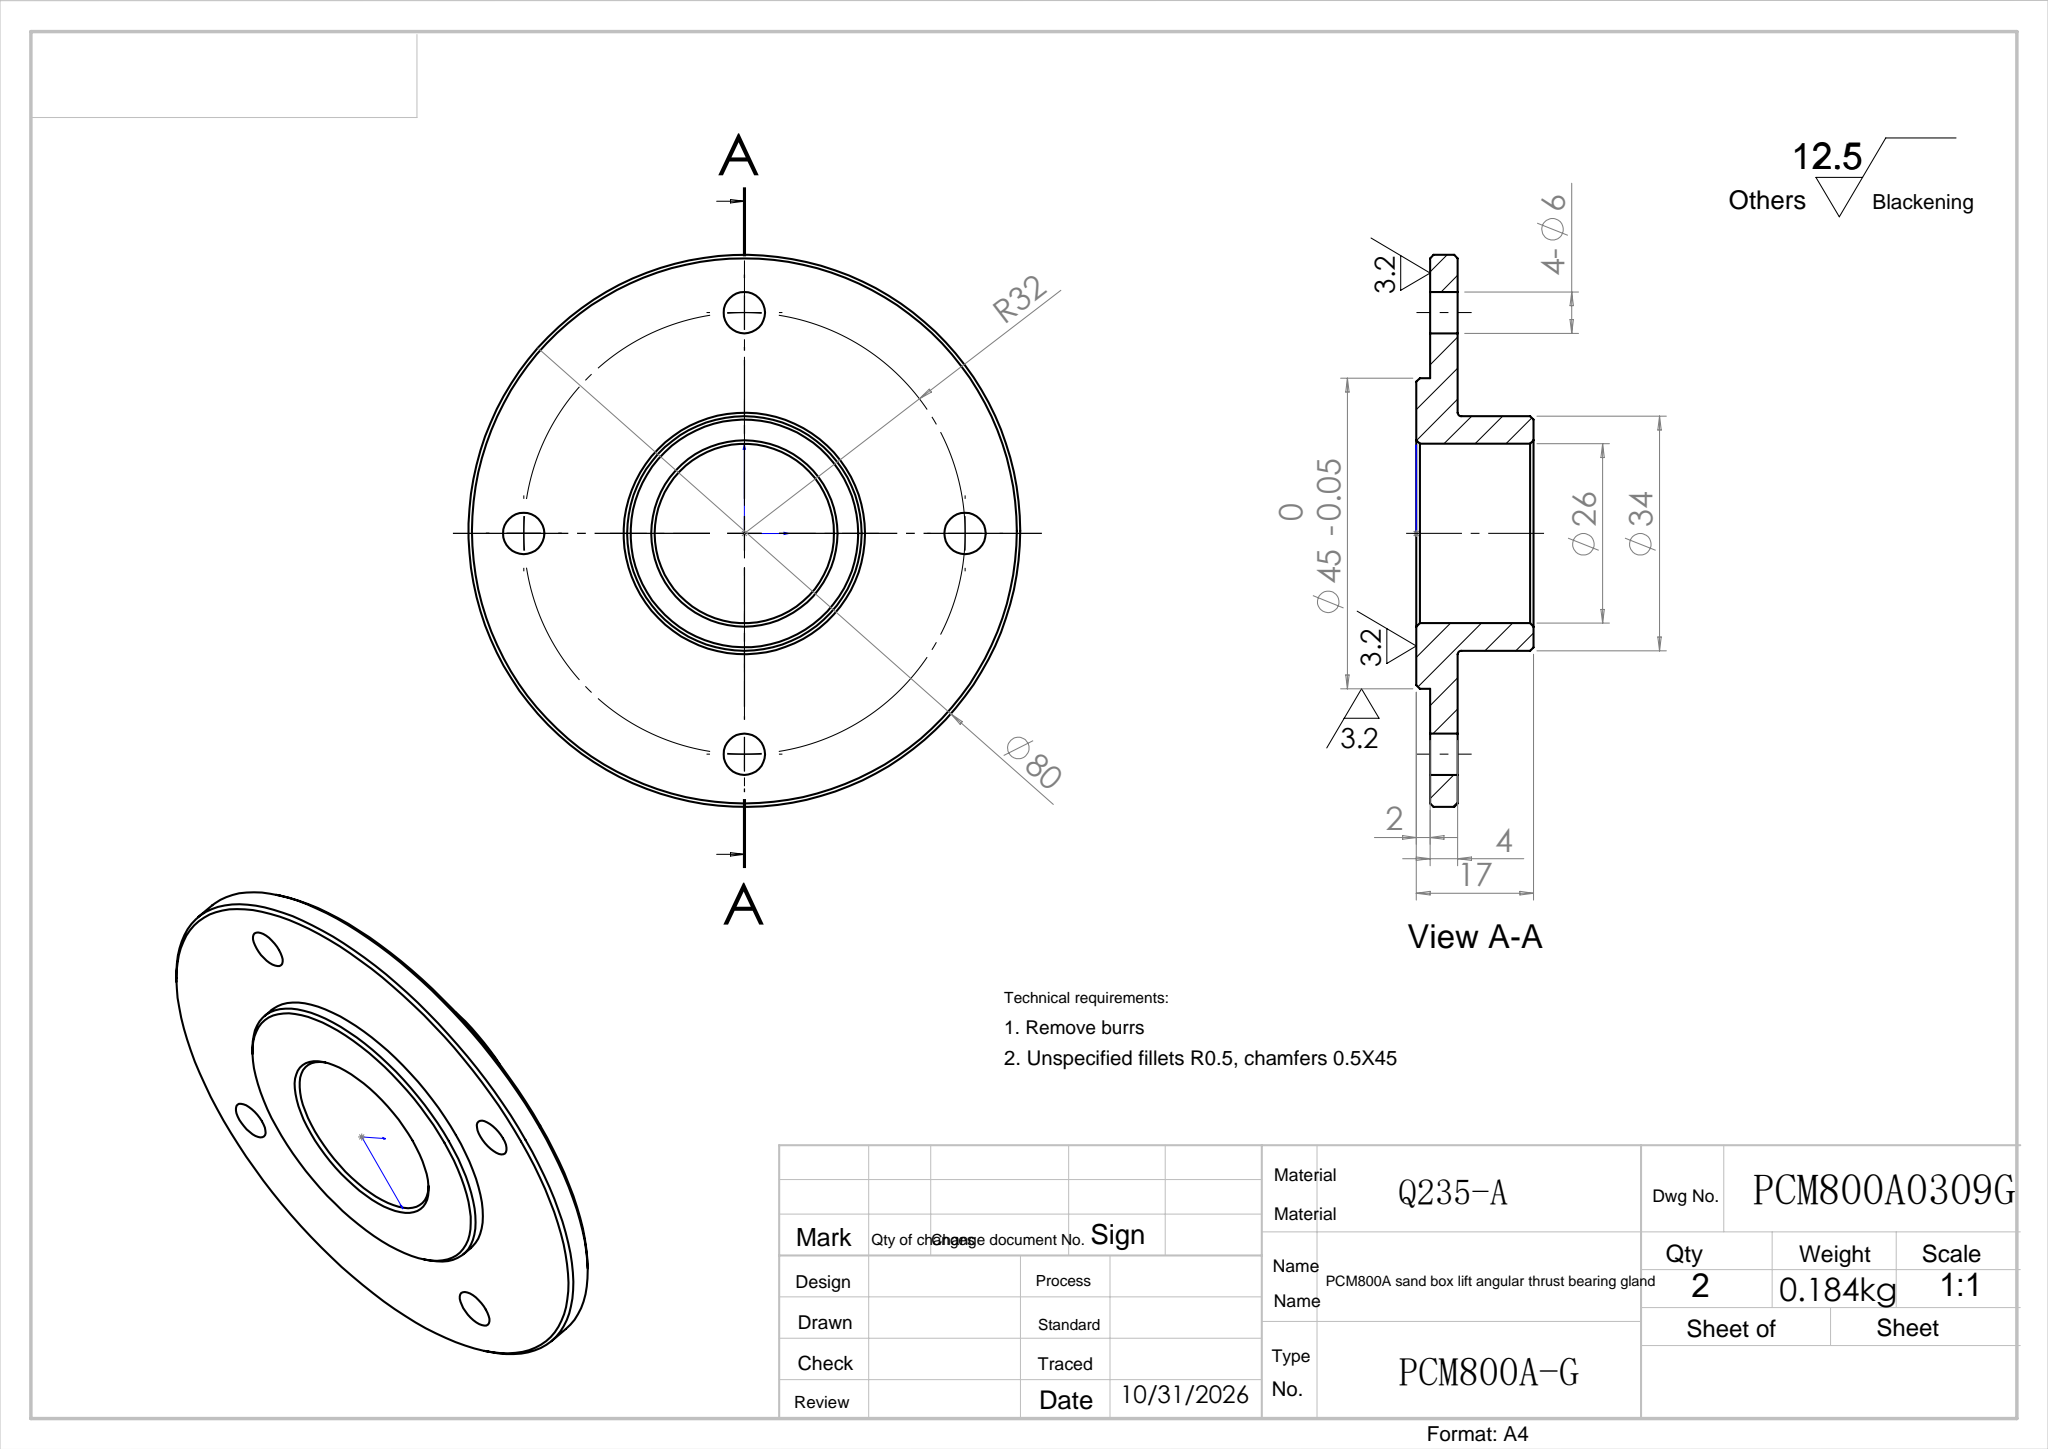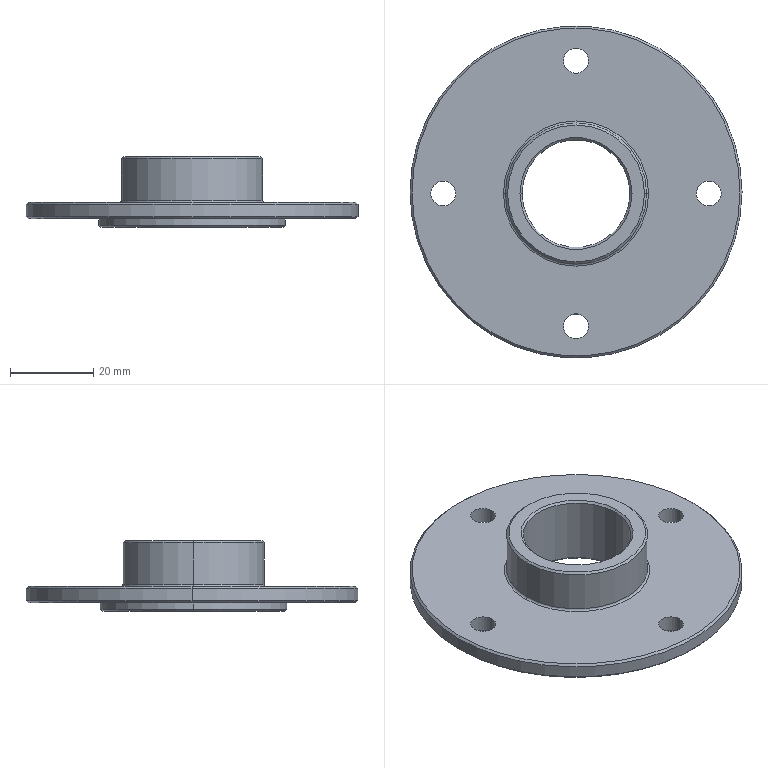Part | SolidWorks | features Boss 2, Chamfer 1, Cut 1, Extrusion 1, Fillet 1 | 1 solid | 34 faces | box 80 x 80 x 17 mm | volume 23688 mm3 | cylinder 16 | cone 12 | plane 4 | torus 2 | commonest cylinder face diameters 6 x8 26 x2 34 x2 45 x2 80 x2
STEP:
#1=CARTESIAN_POINT('',(29.,0.,2.));
#2=VERTEX_POINT('',#1);
#3=CARTESIAN_POINT('',(35.,0.,2.));
#4=VERTEX_POINT('',#3);
#5=CARTESIAN_POINT('',(32.,0.,2.));
#6=DIRECTION('',(0.,0.,1.));
#7=DIRECTION('',(1.,0.,0.));
#8=AXIS2_PLACEMENT_3D('',#5,#6,#7);
#9=CIRCLE('',#8,3.);
#10=EDGE_CURVE('',#2,#4,#9,.T.);
#11=ORIENTED_EDGE('',*,*,#10,.F.);
#12=CARTESIAN_POINT('',(29.,0.,6.));
#13=VERTEX_POINT('',#12);
#14=CARTESIAN_POINT('',(29.,0.,0.));
#15=DIRECTION('',(0.,0.,1.));
#16=VECTOR('',#15,1000.);
#17=LINE('',#14,#16);
#18=EDGE_CURVE('',#2,#13,#17,.T.);
#19=ORIENTED_EDGE('',*,*,#18,.T.);
#20=CARTESIAN_POINT('',(35.,0.,6.));
#21=VERTEX_POINT('',#20);
#22=CARTESIAN_POINT('',(32.,0.,6.));
#23=DIRECTION('',(0.,0.,1.));
#24=DIRECTION('',(1.,0.,0.));
#25=AXIS2_PLACEMENT_3D('',#22,#23,#24);
#26=CIRCLE('',#25,3.);
#27=EDGE_CURVE('',#13,#21,#26,.T.);
#28=ORIENTED_EDGE('',*,*,#27,.T.);
#29=CARTESIAN_POINT('',(35.,0.,0.));
#30=DIRECTION('',(0.,0.,1.));
#31=VECTOR('',#30,1000.);
#32=LINE('',#29,#31);
#33=EDGE_CURVE('',#4,#21,#32,.T.);
#34=ORIENTED_EDGE('',*,*,#33,.F.);
#35=EDGE_LOOP('',(#11,#19,#28,#34));
#36=FACE_OUTER_BOUND('',#35,.T.);
#37=CARTESIAN_POINT('',(32.,0.,0.));
#38=DIRECTION('',(0.,0.,1.));
#39=DIRECTION('',(1.,0.,0.));
#40=AXIS2_PLACEMENT_3D('',#37,#38,#39);
#41=CYLINDRICAL_SURFACE('',#40,3.);
#42=ADVANCED_FACE('',(#36),#41,.F.);
#43=CARTESIAN_POINT('',(-3.,-32.,2.));
#44=VERTEX_POINT('',#43);
#45=CARTESIAN_POINT('',(3.,-32.,2.));
#46=VERTEX_POINT('',#45);
#47=CARTESIAN_POINT('',(0.,-32.,2.));
#48=DIRECTION('',(0.,0.,1.));
#49=DIRECTION('',(1.,0.,0.));
#50=AXIS2_PLACEMENT_3D('',#47,#48,#49);
#51=CIRCLE('',#50,3.);
#52=EDGE_CURVE('',#44,#46,#51,.T.);
#53=ORIENTED_EDGE('',*,*,#52,.F.);
#54=CARTESIAN_POINT('',(-3.,-32.,6.));
#55=VERTEX_POINT('',#54);
#56=CARTESIAN_POINT('',(-3.,-32.,0.));
#57=DIRECTION('',(0.,0.,1.));
#58=VECTOR('',#57,1000.);
#59=LINE('',#56,#58);
#60=EDGE_CURVE('',#44,#55,#59,.T.);
#61=ORIENTED_EDGE('',*,*,#60,.T.);
#62=CARTESIAN_POINT('',(3.,-32.,6.));
#63=VERTEX_POINT('',#62);
#64=CARTESIAN_POINT('',(0.,-32.,6.));
#65=DIRECTION('',(0.,0.,1.));
#66=DIRECTION('',(1.,0.,0.));
#67=AXIS2_PLACEMENT_3D('',#64,#65,#66);
#68=CIRCLE('',#67,3.);
#69=EDGE_CURVE('',#55,#63,#68,.T.);
#70=ORIENTED_EDGE('',*,*,#69,.T.);
#71=CARTESIAN_POINT('',(3.,-32.,0.));
#72=DIRECTION('',(0.,0.,1.));
#73=VECTOR('',#72,1000.);
#74=LINE('',#71,#73);
#75=EDGE_CURVE('',#46,#63,#74,.T.);
#76=ORIENTED_EDGE('',*,*,#75,.F.);
#77=EDGE_LOOP('',(#53,#61,#70,#76));
#78=FACE_OUTER_BOUND('',#77,.T.);
#79=CARTESIAN_POINT('',(0.,-32.,0.));
#80=DIRECTION('',(0.,0.,1.));
#81=DIRECTION('',(1.,0.,0.));
#82=AXIS2_PLACEMENT_3D('',#79,#80,#81);
#83=CYLINDRICAL_SURFACE('',#82,3.);
#84=ADVANCED_FACE('',(#78),#83,.F.);
#85=CARTESIAN_POINT('',(-35.,0.,2.));
#86=VERTEX_POINT('',#85);
#87=CARTESIAN_POINT('',(-29.,0.,2.));
#88=VERTEX_POINT('',#87);
#89=CARTESIAN_POINT('',(-32.,0.,2.));
#90=DIRECTION('',(0.,0.,1.));
#91=DIRECTION('',(1.,0.,0.));
#92=AXIS2_PLACEMENT_3D('',#89,#90,#91);
#93=CIRCLE('',#92,3.);
#94=EDGE_CURVE('',#86,#88,#93,.T.);
#95=ORIENTED_EDGE('',*,*,#94,.F.);
#96=CARTESIAN_POINT('',(-35.,0.,6.));
#97=VERTEX_POINT('',#96);
#98=CARTESIAN_POINT('',(-35.,0.,0.));
#99=DIRECTION('',(0.,0.,1.));
#100=VECTOR('',#99,1000.);
#101=LINE('',#98,#100);
#102=EDGE_CURVE('',#86,#97,#101,.T.);
#103=ORIENTED_EDGE('',*,*,#102,.T.);
#104=CARTESIAN_POINT('',(-29.,0.,6.));
#105=VERTEX_POINT('',#104);
#106=CARTESIAN_POINT('',(-32.,0.,6.));
#107=DIRECTION('',(0.,0.,1.));
#108=DIRECTION('',(1.,0.,0.));
#109=AXIS2_PLACEMENT_3D('',#106,#107,#108);
#110=CIRCLE('',#109,3.);
#111=EDGE_CURVE('',#97,#105,#110,.T.);
#112=ORIENTED_EDGE('',*,*,#111,.T.);
#113=CARTESIAN_POINT('',(-29.,0.,0.));
#114=DIRECTION('',(0.,0.,1.));
#115=VECTOR('',#114,1000.);
#116=LINE('',#113,#115);
#117=EDGE_CURVE('',#88,#105,#116,.T.);
#118=ORIENTED_EDGE('',*,*,#117,.F.);
#119=EDGE_LOOP('',(#95,#103,#112,#118));
#120=FACE_OUTER_BOUND('',#119,.T.);
#121=CARTESIAN_POINT('',(-32.,0.,0.));
#122=DIRECTION('',(0.,0.,1.));
#123=DIRECTION('',(1.,0.,0.));
#124=AXIS2_PLACEMENT_3D('',#121,#122,#123);
#125=CYLINDRICAL_SURFACE('',#124,3.);
#126=ADVANCED_FACE('',(#120),#125,.F.);
#127=CARTESIAN_POINT('',(-3.,32.,2.));
#128=VERTEX_POINT('',#127);
#129=CARTESIAN_POINT('',(3.,32.,2.));
#130=VERTEX_POINT('',#129);
#131=CARTESIAN_POINT('',(0.,32.,2.));
#132=DIRECTION('',(0.,0.,1.));
#133=DIRECTION('',(1.,0.,0.));
#134=AXIS2_PLACEMENT_3D('',#131,#132,#133);
#135=CIRCLE('',#134,3.);
#136=EDGE_CURVE('',#128,#130,#135,.T.);
#137=ORIENTED_EDGE('',*,*,#136,.F.);
#138=CARTESIAN_POINT('',(-3.,32.,6.));
#139=VERTEX_POINT('',#138);
#140=CARTESIAN_POINT('',(-3.,32.,0.));
#141=DIRECTION('',(0.,0.,1.));
#142=VECTOR('',#141,1000.);
#143=LINE('',#140,#142);
#144=EDGE_CURVE('',#128,#139,#143,.T.);
#145=ORIENTED_EDGE('',*,*,#144,.T.);
#146=CARTESIAN_POINT('',(3.,32.,6.));
#147=VERTEX_POINT('',#146);
#148=CARTESIAN_POINT('',(0.,32.,6.));
#149=DIRECTION('',(0.,0.,1.));
#150=DIRECTION('',(1.,0.,0.));
#151=AXIS2_PLACEMENT_3D('',#148,#149,#150);
#152=CIRCLE('',#151,3.);
#153=EDGE_CURVE('',#139,#147,#152,.T.);
#154=ORIENTED_EDGE('',*,*,#153,.T.);
#155=CARTESIAN_POINT('',(3.,32.,0.));
#156=DIRECTION('',(0.,0.,1.));
#157=VECTOR('',#156,1000.);
#158=LINE('',#155,#157);
#159=EDGE_CURVE('',#130,#147,#158,.T.);
#160=ORIENTED_EDGE('',*,*,#159,.F.);
#161=EDGE_LOOP('',(#137,#145,#154,#160));
#162=FACE_OUTER_BOUND('',#161,.T.);
#163=CARTESIAN_POINT('',(0.,32.,0.));
#164=DIRECTION('',(0.,0.,1.));
#165=DIRECTION('',(1.,0.,0.));
#166=AXIS2_PLACEMENT_3D('',#163,#164,#165);
#167=CYLINDRICAL_SURFACE('',#166,3.);
#168=ADVANCED_FACE('',(#162),#167,.F.);
#169=CARTESIAN_POINT('',(-17.,0.,6.5));
#170=VERTEX_POINT('',#169);
#171=CARTESIAN_POINT('',(17.,0.,6.5));
#172=VERTEX_POINT('',#171);
#173=CARTESIAN_POINT('',(0.,0.,6.5));
#174=DIRECTION('',(0.,0.,1.));
#175=DIRECTION('',(1.,0.,0.));
#176=AXIS2_PLACEMENT_3D('',#173,#174,#175);
#177=CIRCLE('',#176,17.);
#178=EDGE_CURVE('',#170,#172,#177,.T.);
#179=ORIENTED_EDGE('',*,*,#178,.F.);
#180=CARTESIAN_POINT('',(-17.5,0.,6.));
#181=VERTEX_POINT('',#180);
#182=CARTESIAN_POINT('',(-17.5,0.,6.5));
#183=DIRECTION('',(0.,1.,0.));
#184=DIRECTION('',(-1.,0.,0.));
#185=AXIS2_PLACEMENT_3D('',#182,#183,#184);
#186=CIRCLE('',#185,0.5);
#187=EDGE_CURVE('',#170,#181,#186,.T.);
#188=ORIENTED_EDGE('',*,*,#187,.T.);
#189=CARTESIAN_POINT('',(17.5,0.,6.));
#190=VERTEX_POINT('',#189);
#191=CARTESIAN_POINT('',(0.,0.,6.));
#192=DIRECTION('',(0.,0.,-1.));
#193=DIRECTION('',(1.,0.,0.));
#194=AXIS2_PLACEMENT_3D('',#191,#192,#193);
#195=CIRCLE('',#194,17.5);
#196=EDGE_CURVE('',#190,#181,#195,.T.);
#197=ORIENTED_EDGE('',*,*,#196,.F.);
#198=CARTESIAN_POINT('',(17.5,0.,6.5));
#199=DIRECTION('',(0.,-1.,0.));
#200=DIRECTION('',(0.,0.,-1.));
#201=AXIS2_PLACEMENT_3D('',#198,#199,#200);
#202=CIRCLE('',#201,0.5);
#203=EDGE_CURVE('',#172,#190,#202,.T.);
#204=ORIENTED_EDGE('',*,*,#203,.F.);
#205=EDGE_LOOP('',(#179,#188,#197,#204));
#206=FACE_OUTER_BOUND('',#205,.T.);
#207=CARTESIAN_POINT('',(0.,0.,6.5));
#208=DIRECTION('',(0.,0.,1.));
#209=DIRECTION('',(1.,0.,0.));
#210=AXIS2_PLACEMENT_3D('',#207,#208,#209);
#211=TOROIDAL_SURFACE('',#210,17.5,0.5);
#212=ADVANCED_FACE('',(#206),#211,.F.);
#213=CARTESIAN_POINT('',(16.5,0.,17.));
#214=VERTEX_POINT('',#213);
#215=CARTESIAN_POINT('',(-16.5,0.,17.));
#216=VERTEX_POINT('',#215);
#217=CARTESIAN_POINT('',(0.,0.,17.));
#218=DIRECTION('',(0.,0.,1.));
#219=DIRECTION('',(1.,0.,0.));
#220=AXIS2_PLACEMENT_3D('',#217,#218,#219);
#221=CIRCLE('',#220,16.5);
#222=EDGE_CURVE('',#214,#216,#221,.T.);
#223=ORIENTED_EDGE('',*,*,#222,.F.);
#224=CARTESIAN_POINT('',(17.,0.,16.5));
#225=VERTEX_POINT('',#224);
#226=CARTESIAN_POINT('',(16.5,0.,17.));
#227=DIRECTION('',(0.7071,0.,-0.7071));
#228=VECTOR('',#227,1000.);
#229=LINE('',#226,#228);
#230=EDGE_CURVE('',#214,#225,#229,.T.);
#231=ORIENTED_EDGE('',*,*,#230,.T.);
#232=CARTESIAN_POINT('',(-17.,0.,16.5));
#233=VERTEX_POINT('',#232);
#234=CARTESIAN_POINT('',(0.,0.,16.5));
#235=DIRECTION('',(0.,0.,-1.));
#236=DIRECTION('',(1.,0.,0.));
#237=AXIS2_PLACEMENT_3D('',#234,#235,#236);
#238=CIRCLE('',#237,17.);
#239=EDGE_CURVE('',#233,#225,#238,.T.);
#240=ORIENTED_EDGE('',*,*,#239,.F.);
#241=CARTESIAN_POINT('',(-16.5,0.,17.));
#242=DIRECTION('',(-0.7071,0.,-0.7071));
#243=VECTOR('',#242,1000.);
#244=LINE('',#241,#243);
#245=EDGE_CURVE('',#216,#233,#244,.T.);
#246=ORIENTED_EDGE('',*,*,#245,.F.);
#247=EDGE_LOOP('',(#223,#231,#240,#246));
#248=FACE_OUTER_BOUND('',#247,.T.);
#249=CARTESIAN_POINT('',(0.,0.,17.));
#250=DIRECTION('',(0.,0.,-1.));
#251=DIRECTION('',(-1.,0.,0.));
#252=AXIS2_PLACEMENT_3D('',#249,#250,#251);
#253=CONICAL_SURFACE('',#252,16.5,0.7854);
#254=ADVANCED_FACE('',(#248),#253,.T.);
#255=CARTESIAN_POINT('',(39.5,0.3744,6.));
#256=VERTEX_POINT('',#255);
#257=CARTESIAN_POINT('',(-39.5,0.3744,6.));
#258=VERTEX_POINT('',#257);
#259=CARTESIAN_POINT('',(0.,0.3744,6.));
#260=DIRECTION('',(0.,0.,1.));
#261=DIRECTION('',(1.,0.,0.));
#262=AXIS2_PLACEMENT_3D('',#259,#260,#261);
#263=CIRCLE('',#262,39.5);
#264=EDGE_CURVE('',#256,#258,#263,.T.);
#265=ORIENTED_EDGE('',*,*,#264,.F.);
#266=CARTESIAN_POINT('',(40.,0.3744,5.5));
#267=VERTEX_POINT('',#266);
#268=CARTESIAN_POINT('',(39.5,0.3744,6.));
#269=DIRECTION('',(0.7071,0.,-0.7071));
#270=VECTOR('',#269,1000.);
#271=LINE('',#268,#270);
#272=EDGE_CURVE('',#256,#267,#271,.T.);
#273=ORIENTED_EDGE('',*,*,#272,.T.);
#274=CARTESIAN_POINT('',(-40.,0.3744,5.5));
#275=VERTEX_POINT('',#274);
#276=CARTESIAN_POINT('',(0.,0.3744,5.5));
#277=DIRECTION('',(0.,0.,-1.));
#278=DIRECTION('',(1.,0.,0.));
#279=AXIS2_PLACEMENT_3D('',#276,#277,#278);
#280=CIRCLE('',#279,40.);
#281=EDGE_CURVE('',#275,#267,#280,.T.);
#282=ORIENTED_EDGE('',*,*,#281,.F.);
#283=CARTESIAN_POINT('',(-39.5,0.3744,6.));
#284=DIRECTION('',(-0.7071,0.,-0.7071));
#285=VECTOR('',#284,1000.);
#286=LINE('',#283,#285);
#287=EDGE_CURVE('',#258,#275,#286,.T.);
#288=ORIENTED_EDGE('',*,*,#287,.F.);
#289=EDGE_LOOP('',(#265,#273,#282,#288));
#290=FACE_OUTER_BOUND('',#289,.T.);
#291=CARTESIAN_POINT('',(0.,0.3744,6.));
#292=DIRECTION('',(0.,0.,-1.));
#293=DIRECTION('',(-1.,0.,0.));
#294=AXIS2_PLACEMENT_3D('',#291,#292,#293);
#295=CONICAL_SURFACE('',#294,39.5,0.7854);
#296=ADVANCED_FACE('',(#290),#295,.T.);
#297=CARTESIAN_POINT('',(-22.,0.,0.));
#298=VERTEX_POINT('',#297);
#299=CARTESIAN_POINT('',(22.,0.,0.));
#300=VERTEX_POINT('',#299);
#301=CARTESIAN_POINT('',(0.,0.,0.));
#302=DIRECTION('',(0.,0.,-1.));
#303=DIRECTION('',(1.,0.,0.));
#304=AXIS2_PLACEMENT_3D('',#301,#302,#303);
#305=CIRCLE('',#304,22.);
#306=EDGE_CURVE('',#298,#300,#305,.T.);
#307=ORIENTED_EDGE('',*,*,#306,.F.);
#308=CARTESIAN_POINT('',(-22.5,0.,0.5));
#309=VERTEX_POINT('',#308);
#310=CARTESIAN_POINT('',(-22.5,0.,0.5));
#311=DIRECTION('',(-0.7071,0.,0.7071));
#312=VECTOR('',#311,1000.);
#313=LINE('',#310,#312);
#314=EDGE_CURVE('',#298,#309,#313,.T.);
#315=ORIENTED_EDGE('',*,*,#314,.T.);
#316=CARTESIAN_POINT('',(22.5,0.,0.5));
#317=VERTEX_POINT('',#316);
#318=CARTESIAN_POINT('',(0.,0.,0.5));
#319=DIRECTION('',(0.,0.,1.));
#320=DIRECTION('',(1.,0.,0.));
#321=AXIS2_PLACEMENT_3D('',#318,#319,#320);
#322=CIRCLE('',#321,22.5);
#323=EDGE_CURVE('',#317,#309,#322,.T.);
#324=ORIENTED_EDGE('',*,*,#323,.F.);
#325=CARTESIAN_POINT('',(22.5,0.,0.5));
#326=DIRECTION('',(0.7071,0.,0.7071));
#327=VECTOR('',#326,1000.);
#328=LINE('',#325,#327);
#329=EDGE_CURVE('',#300,#317,#328,.T.);
#330=ORIENTED_EDGE('',*,*,#329,.F.);
#331=EDGE_LOOP('',(#307,#315,#324,#330));
#332=FACE_OUTER_BOUND('',#331,.T.);
#333=CARTESIAN_POINT('',(0.,0.,0.5));
#334=DIRECTION('',(0.,0.,1.));
#335=DIRECTION('',(1.,0.,0.));
#336=AXIS2_PLACEMENT_3D('',#333,#334,#335);
#337=CONICAL_SURFACE('',#336,22.5,0.7854);
#338=ADVANCED_FACE('',(#332),#337,.T.);
#339=CARTESIAN_POINT('',(13.,0.,0.5));
#340=VERTEX_POINT('',#339);
#341=CARTESIAN_POINT('',(-13.,0.,0.5));
#342=VERTEX_POINT('',#341);
#343=CARTESIAN_POINT('',(0.,0.,0.5));
#344=DIRECTION('',(0.,0.,-1.));
#345=DIRECTION('',(1.,0.,0.));
#346=AXIS2_PLACEMENT_3D('',#343,#344,#345);
#347=CIRCLE('',#346,13.);
#348=EDGE_CURVE('',#340,#342,#347,.T.);
#349=ORIENTED_EDGE('',*,*,#348,.F.);
#350=CARTESIAN_POINT('',(13.5,0.,0.));
#351=VERTEX_POINT('',#350);
#352=CARTESIAN_POINT('',(13.5,0.,0.));
#353=DIRECTION('',(0.7071,0.,-0.7071));
#354=VECTOR('',#353,1000.);
#355=LINE('',#352,#354);
#356=EDGE_CURVE('',#340,#351,#355,.T.);
#357=ORIENTED_EDGE('',*,*,#356,.T.);
#358=CARTESIAN_POINT('',(-13.5,0.,0.));
#359=VERTEX_POINT('',#358);
#360=CARTESIAN_POINT('',(0.,0.,0.));
#361=DIRECTION('',(0.,0.,1.));
#362=DIRECTION('',(1.,0.,0.));
#363=AXIS2_PLACEMENT_3D('',#360,#361,#362);
#364=CIRCLE('',#363,13.5);
#365=EDGE_CURVE('',#359,#351,#364,.T.);
#366=ORIENTED_EDGE('',*,*,#365,.F.);
#367=CARTESIAN_POINT('',(-13.5,0.,0.));
#368=DIRECTION('',(-0.7071,0.,-0.7071));
#369=VECTOR('',#368,1000.);
#370=LINE('',#367,#369);
#371=EDGE_CURVE('',#342,#359,#370,.T.);
#372=ORIENTED_EDGE('',*,*,#371,.F.);
#373=EDGE_LOOP('',(#349,#357,#366,#372));
#374=FACE_OUTER_BOUND('',#373,.T.);
#375=CARTESIAN_POINT('',(0.,0.,0.));
#376=DIRECTION('',(0.,0.,-1.));
#377=DIRECTION('',(-1.,0.,0.));
#378=AXIS2_PLACEMENT_3D('',#375,#376,#377);
#379=CONICAL_SURFACE('',#378,13.5,0.7854);
#380=ADVANCED_FACE('',(#374),#379,.F.);
#381=CARTESIAN_POINT('',(-13.,0.,16.5));
#382=VERTEX_POINT('',#381);
#383=CARTESIAN_POINT('',(13.,0.,16.5));
#384=VERTEX_POINT('',#383);
#385=CARTESIAN_POINT('',(0.,0.,16.5));
#386=DIRECTION('',(0.,0.,1.));
#387=DIRECTION('',(1.,0.,0.));
#388=AXIS2_PLACEMENT_3D('',#385,#386,#387);
#389=CIRCLE('',#388,13.);
#390=EDGE_CURVE('',#382,#384,#389,.T.);
#391=ORIENTED_EDGE('',*,*,#390,.F.);
#392=CARTESIAN_POINT('',(-13.5,0.,17.));
#393=VERTEX_POINT('',#392);
#394=CARTESIAN_POINT('',(-13.,0.,16.5));
#395=DIRECTION('',(-0.7071,0.,0.7071));
#396=VECTOR('',#395,1000.);
#397=LINE('',#394,#396);
#398=EDGE_CURVE('',#382,#393,#397,.T.);
#399=ORIENTED_EDGE('',*,*,#398,.T.);
#400=CARTESIAN_POINT('',(13.5,0.,17.));
#401=VERTEX_POINT('',#400);
#402=CARTESIAN_POINT('',(0.,0.,17.));
#403=DIRECTION('',(0.,0.,-1.));
#404=DIRECTION('',(1.,0.,0.));
#405=AXIS2_PLACEMENT_3D('',#402,#403,#404);
#406=CIRCLE('',#405,13.5);
#407=EDGE_CURVE('',#401,#393,#406,.T.);
#408=ORIENTED_EDGE('',*,*,#407,.F.);
#409=CARTESIAN_POINT('',(13.,0.,16.5));
#410=DIRECTION('',(0.7071,0.,0.7071));
#411=VECTOR('',#410,1000.);
#412=LINE('',#409,#411);
#413=EDGE_CURVE('',#384,#401,#412,.T.);
#414=ORIENTED_EDGE('',*,*,#413,.F.);
#415=EDGE_LOOP('',(#391,#399,#408,#414));
#416=FACE_OUTER_BOUND('',#415,.T.);
#417=CARTESIAN_POINT('',(0.,0.,16.5));
#418=DIRECTION('',(0.,0.,1.));
#419=DIRECTION('',(1.,0.,0.));
#420=AXIS2_PLACEMENT_3D('',#417,#418,#419);
#421=CONICAL_SURFACE('',#420,13.,0.7854);
#422=ADVANCED_FACE('',(#416),#421,.F.);
#423=CARTESIAN_POINT('',(-39.5,0.3744,2.));
#424=VERTEX_POINT('',#423);
#425=CARTESIAN_POINT('',(39.5,0.3744,2.));
#426=VERTEX_POINT('',#425);
#427=CARTESIAN_POINT('',(0.,0.3744,2.));
#428=DIRECTION('',(0.,0.,-1.));
#429=DIRECTION('',(1.,0.,0.));
#430=AXIS2_PLACEMENT_3D('',#427,#428,#429);
#431=CIRCLE('',#430,39.5);
#432=EDGE_CURVE('',#424,#426,#431,.T.);
#433=ORIENTED_EDGE('',*,*,#432,.F.);
#434=CARTESIAN_POINT('',(-40.,0.3744,2.5));
#435=VERTEX_POINT('',#434);
#436=CARTESIAN_POINT('',(-40.,0.3744,2.5));
#437=DIRECTION('',(-0.7071,0.,0.7071));
#438=VECTOR('',#437,1000.);
#439=LINE('',#436,#438);
#440=EDGE_CURVE('',#424,#435,#439,.T.);
#441=ORIENTED_EDGE('',*,*,#440,.T.);
#442=CARTESIAN_POINT('',(40.,0.3744,2.5));
#443=VERTEX_POINT('',#442);
#444=CARTESIAN_POINT('',(0.,0.3744,2.5));
#445=DIRECTION('',(0.,0.,1.));
#446=DIRECTION('',(1.,0.,0.));
#447=AXIS2_PLACEMENT_3D('',#444,#445,#446);
#448=CIRCLE('',#447,40.);
#449=EDGE_CURVE('',#443,#435,#448,.T.);
#450=ORIENTED_EDGE('',*,*,#449,.F.);
#451=CARTESIAN_POINT('',(40.,0.3744,2.5));
#452=DIRECTION('',(0.7071,0.,0.7071));
#453=VECTOR('',#452,1000.);
#454=LINE('',#451,#453);
#455=EDGE_CURVE('',#426,#443,#454,.T.);
#456=ORIENTED_EDGE('',*,*,#455,.F.);
#457=EDGE_LOOP('',(#433,#441,#450,#456));
#458=FACE_OUTER_BOUND('',#457,.T.);
#459=CARTESIAN_POINT('',(0.,0.3744,2.5));
#460=DIRECTION('',(0.,0.,1.));
#461=DIRECTION('',(1.,0.,0.));
#462=AXIS2_PLACEMENT_3D('',#459,#460,#461);
#463=CONICAL_SURFACE('',#462,40.,0.7854);
#464=ADVANCED_FACE('',(#458),#463,.T.);
#465=ORIENTED_EDGE('',*,*,#239,.T.);
#466=CARTESIAN_POINT('',(17.,0.,17.));
#467=DIRECTION('',(0.,0.,-1.));
#468=VECTOR('',#467,1000.);
#469=LINE('',#466,#468);
#470=EDGE_CURVE('',#225,#172,#469,.T.);
#471=ORIENTED_EDGE('',*,*,#470,.T.);
#472=CARTESIAN_POINT('',(0.,0.,6.5));
#473=DIRECTION('',(0.,0.,1.));
#474=DIRECTION('',(1.,0.,0.));
#475=AXIS2_PLACEMENT_3D('',#472,#473,#474);
#476=CIRCLE('',#475,17.);
#477=EDGE_CURVE('',#172,#170,#476,.T.);
#478=ORIENTED_EDGE('',*,*,#477,.T.);
#479=CARTESIAN_POINT('',(-17.,0.,17.));
#480=DIRECTION('',(0.,0.,-1.));
#481=VECTOR('',#480,1000.);
#482=LINE('',#479,#481);
#483=EDGE_CURVE('',#233,#170,#482,.T.);
#484=ORIENTED_EDGE('',*,*,#483,.F.);
#485=EDGE_LOOP('',(#465,#471,#478,#484));
#486=FACE_OUTER_BOUND('',#485,.T.);
#487=CARTESIAN_POINT('',(0.,0.,17.));
#488=DIRECTION('',(0.,0.,-1.));
#489=DIRECTION('',(-1.,0.,0.));
#490=AXIS2_PLACEMENT_3D('',#487,#488,#489);
#491=CYLINDRICAL_SURFACE('',#490,17.);
#492=ADVANCED_FACE('',(#486),#491,.T.);
#493=ORIENTED_EDGE('',*,*,#281,.T.);
#494=CARTESIAN_POINT('',(40.,0.3744,6.));
#495=DIRECTION('',(0.,0.,-1.));
#496=VECTOR('',#495,1000.);
#497=LINE('',#494,#496);
#498=EDGE_CURVE('',#267,#443,#497,.T.);
#499=ORIENTED_EDGE('',*,*,#498,.T.);
#500=ORIENTED_EDGE('',*,*,#449,.T.);
#501=CARTESIAN_POINT('',(-40.,0.3744,6.));
#502=DIRECTION('',(0.,0.,-1.));
#503=VECTOR('',#502,1000.);
#504=LINE('',#501,#503);
#505=EDGE_CURVE('',#275,#435,#504,.T.);
#506=ORIENTED_EDGE('',*,*,#505,.F.);
#507=EDGE_LOOP('',(#493,#499,#500,#506));
#508=FACE_OUTER_BOUND('',#507,.T.);
#509=CARTESIAN_POINT('',(0.,0.3744,6.));
#510=DIRECTION('',(0.,0.,-1.));
#511=DIRECTION('',(-1.,0.,0.));
#512=AXIS2_PLACEMENT_3D('',#509,#510,#511);
#513=CYLINDRICAL_SURFACE('',#512,40.);
#514=ADVANCED_FACE('',(#508),#513,.T.);
#515=ORIENTED_EDGE('',*,*,#390,.T.);
#516=CARTESIAN_POINT('',(13.,0.,2.));
#517=DIRECTION('',(0.,0.,-1.));
#518=VECTOR('',#517,1000.);
#519=LINE('',#516,#518);
#520=EDGE_CURVE('',#384,#340,#519,.T.);
#521=ORIENTED_EDGE('',*,*,#520,.T.);
#522=ORIENTED_EDGE('',*,*,#348,.T.);
#523=CARTESIAN_POINT('',(-13.,0.,2.));
#524=DIRECTION('',(0.,0.,-1.));
#525=VECTOR('',#524,1000.);
#526=LINE('',#523,#525);
#527=EDGE_CURVE('',#382,#342,#526,.T.);
#528=ORIENTED_EDGE('',*,*,#527,.F.);
#529=EDGE_LOOP('',(#515,#521,#522,#528));
#530=FACE_OUTER_BOUND('',#529,.T.);
#531=CARTESIAN_POINT('',(0.,0.,2.));
#532=DIRECTION('',(0.,0.,-1.));
#533=DIRECTION('',(-1.,0.,0.));
#534=AXIS2_PLACEMENT_3D('',#531,#532,#533);
#535=CYLINDRICAL_SURFACE('',#534,13.);
#536=ADVANCED_FACE('',(#530),#535,.F.);
#537=CARTESIAN_POINT('',(22.5,0.,2.));
#538=VERTEX_POINT('',#537);
#539=CARTESIAN_POINT('',(-22.5,0.,2.));
#540=VERTEX_POINT('',#539);
#541=CARTESIAN_POINT('',(0.,0.,2.));
#542=DIRECTION('',(0.,0.,1.));
#543=DIRECTION('',(1.,0.,0.));
#544=AXIS2_PLACEMENT_3D('',#541,#542,#543);
#545=CIRCLE('',#544,22.5);
#546=EDGE_CURVE('',#538,#540,#545,.T.);
#547=ORIENTED_EDGE('',*,*,#546,.F.);
#548=CARTESIAN_POINT('',(22.5,0.,2.));
#549=DIRECTION('',(0.,0.,-1.));
#550=VECTOR('',#549,1000.);
#551=LINE('',#548,#550);
#552=EDGE_CURVE('',#538,#317,#551,.T.);
#553=ORIENTED_EDGE('',*,*,#552,.T.);
#554=ORIENTED_EDGE('',*,*,#323,.T.);
#555=CARTESIAN_POINT('',(-22.5,0.,2.));
#556=DIRECTION('',(0.,0.,-1.));
#557=VECTOR('',#556,1000.);
#558=LINE('',#555,#557);
#559=EDGE_CURVE('',#540,#309,#558,.T.);
#560=ORIENTED_EDGE('',*,*,#559,.F.);
#561=EDGE_LOOP('',(#547,#553,#554,#560));
#562=FACE_OUTER_BOUND('',#561,.T.);
#563=CARTESIAN_POINT('',(0.,0.,2.));
#564=DIRECTION('',(0.,0.,-1.));
#565=DIRECTION('',(-1.,0.,0.));
#566=AXIS2_PLACEMENT_3D('',#563,#564,#565);
#567=CYLINDRICAL_SURFACE('',#566,22.5);
#568=ADVANCED_FACE('',(#562),#567,.T.);
#569=CARTESIAN_POINT('',(32.,0.,6.));
#570=DIRECTION('',(0.,0.,1.));
#571=DIRECTION('',(1.,0.,0.));
#572=AXIS2_PLACEMENT_3D('',#569,#570,#571);
#573=CIRCLE('',#572,3.);
#574=EDGE_CURVE('',#21,#13,#573,.T.);
#575=ORIENTED_EDGE('',*,*,#574,.F.);
#576=ORIENTED_EDGE('',*,*,#27,.F.);
#577=EDGE_LOOP('',(#575,#576));
#578=FACE_BOUND('',#577,.T.);
#579=CARTESIAN_POINT('',(0.,-32.,6.));
#580=DIRECTION('',(0.,0.,1.));
#581=DIRECTION('',(1.,0.,0.));
#582=AXIS2_PLACEMENT_3D('',#579,#580,#581);
#583=CIRCLE('',#582,3.);
#584=EDGE_CURVE('',#63,#55,#583,.T.);
#585=ORIENTED_EDGE('',*,*,#584,.F.);
#586=ORIENTED_EDGE('',*,*,#69,.F.);
#587=EDGE_LOOP('',(#585,#586));
#588=FACE_BOUND('',#587,.T.);
#589=CARTESIAN_POINT('',(-32.,0.,6.));
#590=DIRECTION('',(0.,0.,1.));
#591=DIRECTION('',(1.,0.,0.));
#592=AXIS2_PLACEMENT_3D('',#589,#590,#591);
#593=CIRCLE('',#592,3.);
#594=EDGE_CURVE('',#105,#97,#593,.T.);
#595=ORIENTED_EDGE('',*,*,#594,.F.);
#596=ORIENTED_EDGE('',*,*,#111,.F.);
#597=EDGE_LOOP('',(#595,#596));
#598=FACE_BOUND('',#597,.T.);
#599=CARTESIAN_POINT('',(0.,32.,6.));
#600=DIRECTION('',(0.,0.,1.));
#601=DIRECTION('',(1.,0.,0.));
#602=AXIS2_PLACEMENT_3D('',#599,#600,#601);
#603=CIRCLE('',#602,3.);
#604=EDGE_CURVE('',#147,#139,#603,.T.);
#605=ORIENTED_EDGE('',*,*,#604,.F.);
#606=ORIENTED_EDGE('',*,*,#153,.F.);
#607=EDGE_LOOP('',(#605,#606));
#608=FACE_BOUND('',#607,.T.);
#609=ORIENTED_EDGE('',*,*,#196,.T.);
#610=CARTESIAN_POINT('',(0.,0.,6.));
#611=DIRECTION('',(0.,0.,-1.));
#612=DIRECTION('',(1.,0.,0.));
#613=AXIS2_PLACEMENT_3D('',#610,#611,#612);
#614=CIRCLE('',#613,17.5);
#615=EDGE_CURVE('',#181,#190,#614,.T.);
#616=ORIENTED_EDGE('',*,*,#615,.T.);
#617=EDGE_LOOP('',(#609,#616));
#618=FACE_BOUND('',#617,.T.);
#619=CARTESIAN_POINT('',(0.,0.3744,6.));
#620=DIRECTION('',(0.,0.,1.));
#621=DIRECTION('',(1.,0.,0.));
#622=AXIS2_PLACEMENT_3D('',#619,#620,#621);
#623=CIRCLE('',#622,39.5);
#624=EDGE_CURVE('',#258,#256,#623,.T.);
#625=ORIENTED_EDGE('',*,*,#624,.T.);
#626=ORIENTED_EDGE('',*,*,#264,.T.);
#627=EDGE_LOOP('',(#625,#626));
#628=FACE_OUTER_BOUND('',#627,.T.);
#629=CARTESIAN_POINT('',(0.,0.3744,6.));
#630=DIRECTION('',(0.,0.,1.));
#631=DIRECTION('',(1.,0.,0.));
#632=AXIS2_PLACEMENT_3D('',#629,#630,#631);
#633=PLANE('',#632);
#634=ADVANCED_FACE('',(#578,#588,#598,#608,#618,#628),#633,.T.);
#635=ORIENTED_EDGE('',*,*,#365,.T.);
#636=CARTESIAN_POINT('',(0.,0.,0.));
#637=DIRECTION('',(0.,0.,1.));
#638=DIRECTION('',(1.,0.,0.));
#639=AXIS2_PLACEMENT_3D('',#636,#637,#638);
#640=CIRCLE('',#639,13.5);
#641=EDGE_CURVE('',#351,#359,#640,.T.);
#642=ORIENTED_EDGE('',*,*,#641,.T.);
#643=EDGE_LOOP('',(#635,#642));
#644=FACE_BOUND('',#643,.T.);
#645=CARTESIAN_POINT('',(0.,0.,0.));
#646=DIRECTION('',(0.,0.,-1.));
#647=DIRECTION('',(1.,0.,0.));
#648=AXIS2_PLACEMENT_3D('',#645,#646,#647);
#649=CIRCLE('',#648,22.);
#650=EDGE_CURVE('',#300,#298,#649,.T.);
#651=ORIENTED_EDGE('',*,*,#650,.T.);
#652=ORIENTED_EDGE('',*,*,#306,.T.);
#653=EDGE_LOOP('',(#651,#652));
#654=FACE_OUTER_BOUND('',#653,.T.);
#655=CARTESIAN_POINT('',(0.,0.,0.));
#656=DIRECTION('',(0.,0.,1.));
#657=DIRECTION('',(1.,0.,0.));
#658=AXIS2_PLACEMENT_3D('',#655,#656,#657);
#659=PLANE('',#658);
#660=ADVANCED_FACE('',(#644,#654),#659,.F.);
#661=ORIENTED_EDGE('',*,*,#552,.F.);
#662=CARTESIAN_POINT('',(0.,0.,2.));
#663=DIRECTION('',(0.,0.,1.));
#664=DIRECTION('',(1.,0.,0.));
#665=AXIS2_PLACEMENT_3D('',#662,#663,#664);
#666=CIRCLE('',#665,22.5);
#667=EDGE_CURVE('',#540,#538,#666,.T.);
#668=ORIENTED_EDGE('',*,*,#667,.F.);
#669=ORIENTED_EDGE('',*,*,#559,.T.);
#670=CARTESIAN_POINT('',(0.,0.,0.5));
#671=DIRECTION('',(0.,0.,1.));
#672=DIRECTION('',(1.,0.,0.));
#673=AXIS2_PLACEMENT_3D('',#670,#671,#672);
#674=CIRCLE('',#673,22.5);
#675=EDGE_CURVE('',#309,#317,#674,.T.);
#676=ORIENTED_EDGE('',*,*,#675,.T.);
#677=EDGE_LOOP('',(#661,#668,#669,#676));
#678=FACE_OUTER_BOUND('',#677,.T.);
#679=CARTESIAN_POINT('',(0.,0.,2.));
#680=DIRECTION('',(0.,0.,-1.));
#681=DIRECTION('',(-1.,0.,0.));
#682=AXIS2_PLACEMENT_3D('',#679,#680,#681);
#683=CYLINDRICAL_SURFACE('',#682,22.5);
#684=ADVANCED_FACE('',(#678),#683,.T.);
#685=ORIENTED_EDGE('',*,*,#520,.F.);
#686=CARTESIAN_POINT('',(0.,0.,16.5));
#687=DIRECTION('',(0.,0.,1.));
#688=DIRECTION('',(1.,0.,0.));
#689=AXIS2_PLACEMENT_3D('',#686,#687,#688);
#690=CIRCLE('',#689,13.);
#691=EDGE_CURVE('',#384,#382,#690,.T.);
#692=ORIENTED_EDGE('',*,*,#691,.T.);
#693=ORIENTED_EDGE('',*,*,#527,.T.);
#694=CARTESIAN_POINT('',(0.,0.,0.5));
#695=DIRECTION('',(0.,0.,-1.));
#696=DIRECTION('',(1.,0.,0.));
#697=AXIS2_PLACEMENT_3D('',#694,#695,#696);
#698=CIRCLE('',#697,13.);
#699=EDGE_CURVE('',#342,#340,#698,.T.);
#700=ORIENTED_EDGE('',*,*,#699,.T.);
#701=EDGE_LOOP('',(#685,#692,#693,#700));
#702=FACE_OUTER_BOUND('',#701,.T.);
#703=CARTESIAN_POINT('',(0.,0.,2.));
#704=DIRECTION('',(0.,0.,-1.));
#705=DIRECTION('',(-1.,0.,0.));
#706=AXIS2_PLACEMENT_3D('',#703,#704,#705);
#707=CYLINDRICAL_SURFACE('',#706,13.);
#708=ADVANCED_FACE('',(#702),#707,.F.);
#709=CARTESIAN_POINT('',(32.,0.,2.));
#710=DIRECTION('',(0.,0.,1.));
#711=DIRECTION('',(1.,0.,0.));
#712=AXIS2_PLACEMENT_3D('',#709,#710,#711);
#713=CIRCLE('',#712,3.);
#714=EDGE_CURVE('',#4,#2,#713,.T.);
#715=ORIENTED_EDGE('',*,*,#714,.T.);
#716=ORIENTED_EDGE('',*,*,#10,.T.);
#717=EDGE_LOOP('',(#715,#716));
#718=FACE_BOUND('',#717,.T.);
#719=CARTESIAN_POINT('',(0.,-32.,2.));
#720=DIRECTION('',(0.,0.,1.));
#721=DIRECTION('',(1.,0.,0.));
#722=AXIS2_PLACEMENT_3D('',#719,#720,#721);
#723=CIRCLE('',#722,3.);
#724=EDGE_CURVE('',#46,#44,#723,.T.);
#725=ORIENTED_EDGE('',*,*,#724,.T.);
#726=ORIENTED_EDGE('',*,*,#52,.T.);
#727=EDGE_LOOP('',(#725,#726));
#728=FACE_BOUND('',#727,.T.);
#729=CARTESIAN_POINT('',(-32.,0.,2.));
#730=DIRECTION('',(0.,0.,1.));
#731=DIRECTION('',(1.,0.,0.));
#732=AXIS2_PLACEMENT_3D('',#729,#730,#731);
#733=CIRCLE('',#732,3.);
#734=EDGE_CURVE('',#88,#86,#733,.T.);
#735=ORIENTED_EDGE('',*,*,#734,.T.);
#736=ORIENTED_EDGE('',*,*,#94,.T.);
#737=EDGE_LOOP('',(#735,#736));
#738=FACE_BOUND('',#737,.T.);
#739=CARTESIAN_POINT('',(0.,32.,2.));
#740=DIRECTION('',(0.,0.,1.));
#741=DIRECTION('',(1.,0.,0.));
#742=AXIS2_PLACEMENT_3D('',#739,#740,#741);
#743=CIRCLE('',#742,3.);
#744=EDGE_CURVE('',#130,#128,#743,.T.);
#745=ORIENTED_EDGE('',*,*,#744,.T.);
#746=ORIENTED_EDGE('',*,*,#136,.T.);
#747=EDGE_LOOP('',(#745,#746));
#748=FACE_BOUND('',#747,.T.);
#749=CARTESIAN_POINT('',(0.,0.3744,2.));
#750=DIRECTION('',(0.,0.,-1.));
#751=DIRECTION('',(1.,0.,0.));
#752=AXIS2_PLACEMENT_3D('',#749,#750,#751);
#753=CIRCLE('',#752,39.5);
#754=EDGE_CURVE('',#426,#424,#753,.T.);
#755=ORIENTED_EDGE('',*,*,#754,.T.);
#756=ORIENTED_EDGE('',*,*,#432,.T.);
#757=EDGE_LOOP('',(#755,#756));
#758=FACE_OUTER_BOUND('',#757,.T.);
#759=ORIENTED_EDGE('',*,*,#667,.T.);
#760=ORIENTED_EDGE('',*,*,#546,.T.);
#761=EDGE_LOOP('',(#759,#760));
#762=FACE_BOUND('',#761,.T.);
#763=CARTESIAN_POINT('',(0.,0.3744,2.));
#764=DIRECTION('',(0.,0.,1.));
#765=DIRECTION('',(1.,0.,0.));
#766=AXIS2_PLACEMENT_3D('',#763,#764,#765);
#767=PLANE('',#766);
#768=ADVANCED_FACE('',(#718,#728,#738,#748,#758,#762),#767,.F.);
#769=ORIENTED_EDGE('',*,*,#498,.F.);
#770=CARTESIAN_POINT('',(0.,0.3744,5.5));
#771=DIRECTION('',(0.,0.,-1.));
#772=DIRECTION('',(1.,0.,0.));
#773=AXIS2_PLACEMENT_3D('',#770,#771,#772);
#774=CIRCLE('',#773,40.);
#775=EDGE_CURVE('',#267,#275,#774,.T.);
#776=ORIENTED_EDGE('',*,*,#775,.T.);
#777=ORIENTED_EDGE('',*,*,#505,.T.);
#778=CARTESIAN_POINT('',(0.,0.3744,2.5));
#779=DIRECTION('',(0.,0.,1.));
#780=DIRECTION('',(1.,0.,0.));
#781=AXIS2_PLACEMENT_3D('',#778,#779,#780);
#782=CIRCLE('',#781,40.);
#783=EDGE_CURVE('',#435,#443,#782,.T.);
#784=ORIENTED_EDGE('',*,*,#783,.T.);
#785=EDGE_LOOP('',(#769,#776,#777,#784));
#786=FACE_OUTER_BOUND('',#785,.T.);
#787=CARTESIAN_POINT('',(0.,0.3744,6.));
#788=DIRECTION('',(0.,0.,-1.));
#789=DIRECTION('',(-1.,0.,0.));
#790=AXIS2_PLACEMENT_3D('',#787,#788,#789);
#791=CYLINDRICAL_SURFACE('',#790,40.);
#792=ADVANCED_FACE('',(#786),#791,.T.);
#793=ORIENTED_EDGE('',*,*,#407,.T.);
#794=CARTESIAN_POINT('',(0.,0.,17.));
#795=DIRECTION('',(0.,0.,-1.));
#796=DIRECTION('',(1.,0.,0.));
#797=AXIS2_PLACEMENT_3D('',#794,#795,#796);
#798=CIRCLE('',#797,13.5);
#799=EDGE_CURVE('',#393,#401,#798,.T.);
#800=ORIENTED_EDGE('',*,*,#799,.T.);
#801=EDGE_LOOP('',(#793,#800));
#802=FACE_BOUND('',#801,.T.);
#803=CARTESIAN_POINT('',(0.,0.,17.));
#804=DIRECTION('',(0.,0.,1.));
#805=DIRECTION('',(1.,0.,0.));
#806=AXIS2_PLACEMENT_3D('',#803,#804,#805);
#807=CIRCLE('',#806,16.5);
#808=EDGE_CURVE('',#216,#214,#807,.T.);
#809=ORIENTED_EDGE('',*,*,#808,.T.);
#810=ORIENTED_EDGE('',*,*,#222,.T.);
#811=EDGE_LOOP('',(#809,#810));
#812=FACE_OUTER_BOUND('',#811,.T.);
#813=CARTESIAN_POINT('',(0.,0.,17.));
#814=DIRECTION('',(0.,0.,1.));
#815=DIRECTION('',(1.,0.,0.));
#816=AXIS2_PLACEMENT_3D('',#813,#814,#815);
#817=PLANE('',#816);
#818=ADVANCED_FACE('',(#802,#812),#817,.T.);
#819=ORIENTED_EDGE('',*,*,#470,.F.);
#820=CARTESIAN_POINT('',(0.,0.,16.5));
#821=DIRECTION('',(0.,0.,-1.));
#822=DIRECTION('',(1.,0.,0.));
#823=AXIS2_PLACEMENT_3D('',#820,#821,#822);
#824=CIRCLE('',#823,17.);
#825=EDGE_CURVE('',#225,#233,#824,.T.);
#826=ORIENTED_EDGE('',*,*,#825,.T.);
#827=ORIENTED_EDGE('',*,*,#483,.T.);
#828=ORIENTED_EDGE('',*,*,#178,.T.);
#829=EDGE_LOOP('',(#819,#826,#827,#828));
#830=FACE_OUTER_BOUND('',#829,.T.);
#831=CARTESIAN_POINT('',(0.,0.,17.));
#832=DIRECTION('',(0.,0.,-1.));
#833=DIRECTION('',(-1.,0.,0.));
#834=AXIS2_PLACEMENT_3D('',#831,#832,#833);
#835=CYLINDRICAL_SURFACE('',#834,17.);
#836=ADVANCED_FACE('',(#830),#835,.T.);
#837=ORIENTED_EDGE('',*,*,#440,.F.);
#838=ORIENTED_EDGE('',*,*,#754,.F.);
#839=ORIENTED_EDGE('',*,*,#455,.T.);
#840=ORIENTED_EDGE('',*,*,#783,.F.);
#841=EDGE_LOOP('',(#837,#838,#839,#840));
#842=FACE_OUTER_BOUND('',#841,.T.);
#843=CARTESIAN_POINT('',(0.,0.3744,2.5));
#844=DIRECTION('',(0.,0.,1.));
#845=DIRECTION('',(1.,0.,0.));
#846=AXIS2_PLACEMENT_3D('',#843,#844,#845);
#847=CONICAL_SURFACE('',#846,40.,0.7854);
#848=ADVANCED_FACE('',(#842),#847,.T.);
#849=ORIENTED_EDGE('',*,*,#398,.F.);
#850=ORIENTED_EDGE('',*,*,#691,.F.);
#851=ORIENTED_EDGE('',*,*,#413,.T.);
#852=ORIENTED_EDGE('',*,*,#799,.F.);
#853=EDGE_LOOP('',(#849,#850,#851,#852));
#854=FACE_OUTER_BOUND('',#853,.T.);
#855=CARTESIAN_POINT('',(0.,0.,16.5));
#856=DIRECTION('',(0.,0.,1.));
#857=DIRECTION('',(1.,0.,0.));
#858=AXIS2_PLACEMENT_3D('',#855,#856,#857);
#859=CONICAL_SURFACE('',#858,13.,0.7854);
#860=ADVANCED_FACE('',(#854),#859,.F.);
#861=ORIENTED_EDGE('',*,*,#356,.F.);
#862=ORIENTED_EDGE('',*,*,#699,.F.);
#863=ORIENTED_EDGE('',*,*,#371,.T.);
#864=ORIENTED_EDGE('',*,*,#641,.F.);
#865=EDGE_LOOP('',(#861,#862,#863,#864));
#866=FACE_OUTER_BOUND('',#865,.T.);
#867=CARTESIAN_POINT('',(0.,0.,0.));
#868=DIRECTION('',(0.,0.,-1.));
#869=DIRECTION('',(-1.,0.,0.));
#870=AXIS2_PLACEMENT_3D('',#867,#868,#869);
#871=CONICAL_SURFACE('',#870,13.5,0.7854);
#872=ADVANCED_FACE('',(#866),#871,.F.);
#873=ORIENTED_EDGE('',*,*,#314,.F.);
#874=ORIENTED_EDGE('',*,*,#650,.F.);
#875=ORIENTED_EDGE('',*,*,#329,.T.);
#876=ORIENTED_EDGE('',*,*,#675,.F.);
#877=EDGE_LOOP('',(#873,#874,#875,#876));
#878=FACE_OUTER_BOUND('',#877,.T.);
#879=CARTESIAN_POINT('',(0.,0.,0.5));
#880=DIRECTION('',(0.,0.,1.));
#881=DIRECTION('',(1.,0.,0.));
#882=AXIS2_PLACEMENT_3D('',#879,#880,#881);
#883=CONICAL_SURFACE('',#882,22.5,0.7854);
#884=ADVANCED_FACE('',(#878),#883,.T.);
#885=ORIENTED_EDGE('',*,*,#272,.F.);
#886=ORIENTED_EDGE('',*,*,#624,.F.);
#887=ORIENTED_EDGE('',*,*,#287,.T.);
#888=ORIENTED_EDGE('',*,*,#775,.F.);
#889=EDGE_LOOP('',(#885,#886,#887,#888));
#890=FACE_OUTER_BOUND('',#889,.T.);
#891=CARTESIAN_POINT('',(0.,0.3744,6.));
#892=DIRECTION('',(0.,0.,-1.));
#893=DIRECTION('',(-1.,0.,0.));
#894=AXIS2_PLACEMENT_3D('',#891,#892,#893);
#895=CONICAL_SURFACE('',#894,39.5,0.7854);
#896=ADVANCED_FACE('',(#890),#895,.T.);
#897=ORIENTED_EDGE('',*,*,#230,.F.);
#898=ORIENTED_EDGE('',*,*,#808,.F.);
#899=ORIENTED_EDGE('',*,*,#245,.T.);
#900=ORIENTED_EDGE('',*,*,#825,.F.);
#901=EDGE_LOOP('',(#897,#898,#899,#900));
#902=FACE_OUTER_BOUND('',#901,.T.);
#903=CARTESIAN_POINT('',(0.,0.,17.));
#904=DIRECTION('',(0.,0.,-1.));
#905=DIRECTION('',(-1.,0.,0.));
#906=AXIS2_PLACEMENT_3D('',#903,#904,#905);
#907=CONICAL_SURFACE('',#906,16.5,0.7854);
#908=ADVANCED_FACE('',(#902),#907,.T.);
#909=ORIENTED_EDGE('',*,*,#187,.F.);
#910=ORIENTED_EDGE('',*,*,#477,.F.);
#911=ORIENTED_EDGE('',*,*,#203,.T.);
#912=ORIENTED_EDGE('',*,*,#615,.F.);
#913=EDGE_LOOP('',(#909,#910,#911,#912));
#914=FACE_OUTER_BOUND('',#913,.T.);
#915=CARTESIAN_POINT('',(0.,0.,6.5));
#916=DIRECTION('',(0.,0.,1.));
#917=DIRECTION('',(1.,0.,0.));
#918=AXIS2_PLACEMENT_3D('',#915,#916,#917);
#919=TOROIDAL_SURFACE('',#918,17.5,0.5);
#920=ADVANCED_FACE('',(#914),#919,.F.);
#921=ORIENTED_EDGE('',*,*,#144,.F.);
#922=ORIENTED_EDGE('',*,*,#744,.F.);
#923=ORIENTED_EDGE('',*,*,#159,.T.);
#924=ORIENTED_EDGE('',*,*,#604,.T.);
#925=EDGE_LOOP('',(#921,#922,#923,#924));
#926=FACE_OUTER_BOUND('',#925,.T.);
#927=CARTESIAN_POINT('',(0.,32.,0.));
#928=DIRECTION('',(0.,0.,1.));
#929=DIRECTION('',(1.,0.,0.));
#930=AXIS2_PLACEMENT_3D('',#927,#928,#929);
#931=CYLINDRICAL_SURFACE('',#930,3.);
#932=ADVANCED_FACE('',(#926),#931,.F.);
#933=ORIENTED_EDGE('',*,*,#102,.F.);
#934=ORIENTED_EDGE('',*,*,#734,.F.);
#935=ORIENTED_EDGE('',*,*,#117,.T.);
#936=ORIENTED_EDGE('',*,*,#594,.T.);
#937=EDGE_LOOP('',(#933,#934,#935,#936));
#938=FACE_OUTER_BOUND('',#937,.T.);
#939=CARTESIAN_POINT('',(-32.,0.,0.));
#940=DIRECTION('',(0.,0.,1.));
#941=DIRECTION('',(1.,0.,0.));
#942=AXIS2_PLACEMENT_3D('',#939,#940,#941);
#943=CYLINDRICAL_SURFACE('',#942,3.);
#944=ADVANCED_FACE('',(#938),#943,.F.);
#945=ORIENTED_EDGE('',*,*,#60,.F.);
#946=ORIENTED_EDGE('',*,*,#724,.F.);
#947=ORIENTED_EDGE('',*,*,#75,.T.);
#948=ORIENTED_EDGE('',*,*,#584,.T.);
#949=EDGE_LOOP('',(#945,#946,#947,#948));
#950=FACE_OUTER_BOUND('',#949,.T.);
#951=CARTESIAN_POINT('',(0.,-32.,0.));
#952=DIRECTION('',(0.,0.,1.));
#953=DIRECTION('',(1.,0.,0.));
#954=AXIS2_PLACEMENT_3D('',#951,#952,#953);
#955=CYLINDRICAL_SURFACE('',#954,3.);
#956=ADVANCED_FACE('',(#950),#955,.F.);
#957=ORIENTED_EDGE('',*,*,#18,.F.);
#958=ORIENTED_EDGE('',*,*,#714,.F.);
#959=ORIENTED_EDGE('',*,*,#33,.T.);
#960=ORIENTED_EDGE('',*,*,#574,.T.);
#961=EDGE_LOOP('',(#957,#958,#959,#960));
#962=FACE_OUTER_BOUND('',#961,.T.);
#963=CARTESIAN_POINT('',(32.,0.,0.));
#964=DIRECTION('',(0.,0.,1.));
#965=DIRECTION('',(1.,0.,0.));
#966=AXIS2_PLACEMENT_3D('',#963,#964,#965);
#967=CYLINDRICAL_SURFACE('',#966,3.);
#968=ADVANCED_FACE('',(#962),#967,.F.);
#969=CLOSED_SHELL('',(#42,#84,#126,#168,#212,#254,#296,#338,#380,#422,#464,#492,#514,#536,#568,#634,#660,#684,#708,#768,#792,#818,#836,#848,#860,#872,#884,#896,#908,#920,#932,#944,#956,#968));
#970=MANIFOLD_SOLID_BREP('',#969);
#971=CARTESIAN_POINT('',(0.,0.,0.));
#972=DIRECTION('',(0.,0.,1.));
#973=DIRECTION('',(1.,0.,0.));
#974=AXIS2_PLACEMENT_3D('',#971,#972,#973);
#975=(LENGTH_UNIT()NAMED_UNIT(*)SI_UNIT(.MILLI.,.METRE.));
#976=UNCERTAINTY_MEASURE_WITH_UNIT(LENGTH_MEASURE(0.00001),#975,'','');
#977=(NAMED_UNIT(*)PLANE_ANGLE_UNIT()SI_UNIT($,.RADIAN.));
#978=(NAMED_UNIT(*)SI_UNIT($,.STERADIAN.)SOLID_ANGLE_UNIT());
#979=(GEOMETRIC_REPRESENTATION_CONTEXT(3)GLOBAL_UNCERTAINTY_ASSIGNED_CONTEXT((#976))GLOBAL_UNIT_ASSIGNED_CONTEXT((#975,#977,#978))REPRESENTATION_CONTEXT('',''));
#980=ADVANCED_BREP_SHAPE_REPRESENTATION('',(#970,#974),#979);